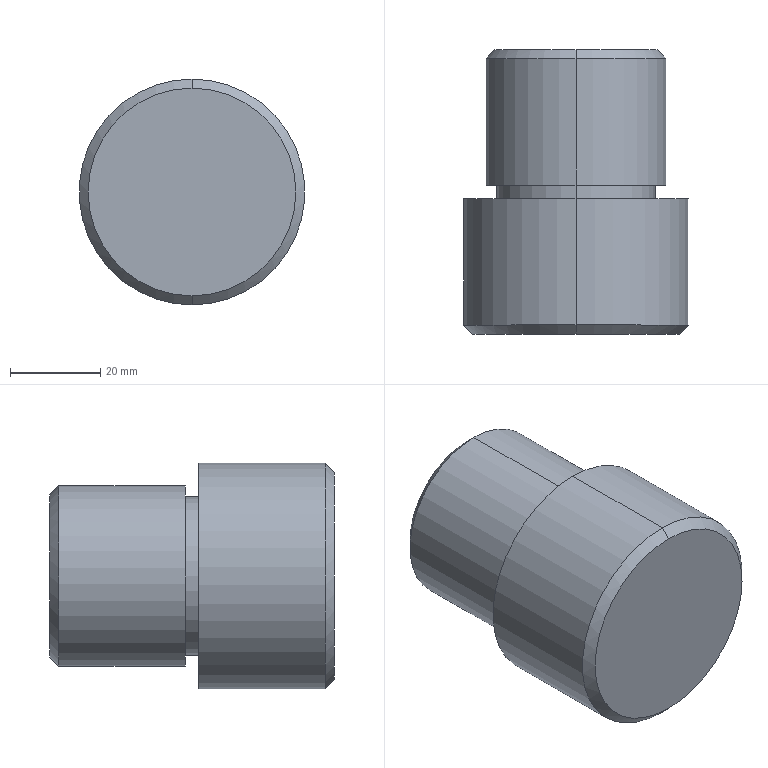Part | SolidWorks | features Chamfer 2, Revolution 1 | 1 solid | 14 faces | box 50 x 63 x 50 mm | volume 98942 mm3 | cylinder 6 | cone 4 | plane 4 | commonest cylinder face diameters 35 x2 40 x2 50 x2
STEP:
#1=CARTESIAN_POINT('',(0.,-35.605,-23.));
#2=VERTEX_POINT('',#1);
#3=CARTESIAN_POINT('',(0.,-35.605,23.));
#4=VERTEX_POINT('',#3);
#5=CARTESIAN_POINT('',(0.,-35.605,0.));
#6=DIRECTION('',(0.,-1.,0.));
#7=DIRECTION('',(0.,0.,1.));
#8=AXIS2_PLACEMENT_3D('',#5,#6,#7);
#9=CIRCLE('',#8,23.);
#10=EDGE_CURVE('',#2,#4,#9,.T.);
#11=ORIENTED_EDGE('',*,*,#10,.F.);
#12=CARTESIAN_POINT('',(0.,-33.605,-25.));
#13=VERTEX_POINT('',#12);
#14=CARTESIAN_POINT('',(0.,-33.605,-25.));
#15=DIRECTION('',(0.,0.7071,-0.7071));
#16=VECTOR('',#15,1000.);
#17=LINE('',#14,#16);
#18=EDGE_CURVE('',#2,#13,#17,.T.);
#19=ORIENTED_EDGE('',*,*,#18,.T.);
#20=CARTESIAN_POINT('',(0.,-33.605,25.));
#21=VERTEX_POINT('',#20);
#22=CARTESIAN_POINT('',(0.,-33.605,0.));
#23=DIRECTION('',(0.,1.,0.));
#24=DIRECTION('',(0.,0.,1.));
#25=AXIS2_PLACEMENT_3D('',#22,#23,#24);
#26=CIRCLE('',#25,25.);
#27=EDGE_CURVE('',#21,#13,#26,.T.);
#28=ORIENTED_EDGE('',*,*,#27,.F.);
#29=CARTESIAN_POINT('',(0.,-33.605,25.));
#30=DIRECTION('',(0.,0.7071,0.7071));
#31=VECTOR('',#30,1000.);
#32=LINE('',#29,#31);
#33=EDGE_CURVE('',#4,#21,#32,.T.);
#34=ORIENTED_EDGE('',*,*,#33,.F.);
#35=EDGE_LOOP('',(#11,#19,#28,#34));
#36=FACE_OUTER_BOUND('',#35,.T.);
#37=CARTESIAN_POINT('',(0.,-33.605,0.));
#38=DIRECTION('',(0.,1.,0.));
#39=DIRECTION('',(0.,0.,1.));
#40=AXIS2_PLACEMENT_3D('',#37,#38,#39);
#41=CONICAL_SURFACE('',#40,25.,0.7854);
#42=ADVANCED_FACE('',(#36),#41,.T.);
#43=CARTESIAN_POINT('',(0.,27.395,18.));
#44=VERTEX_POINT('',#43);
#45=CARTESIAN_POINT('',(0.,27.395,-18.));
#46=VERTEX_POINT('',#45);
#47=CARTESIAN_POINT('',(0.,27.395,0.));
#48=DIRECTION('',(0.,1.,0.));
#49=DIRECTION('',(0.,0.,1.));
#50=AXIS2_PLACEMENT_3D('',#47,#48,#49);
#51=CIRCLE('',#50,18.);
#52=EDGE_CURVE('',#44,#46,#51,.T.);
#53=ORIENTED_EDGE('',*,*,#52,.F.);
#54=CARTESIAN_POINT('',(0.,25.395,20.));
#55=VERTEX_POINT('',#54);
#56=CARTESIAN_POINT('',(0.,27.395,18.));
#57=DIRECTION('',(0.,-0.7071,0.7071));
#58=VECTOR('',#57,1000.);
#59=LINE('',#56,#58);
#60=EDGE_CURVE('',#44,#55,#59,.T.);
#61=ORIENTED_EDGE('',*,*,#60,.T.);
#62=CARTESIAN_POINT('',(0.,25.395,-20.));
#63=VERTEX_POINT('',#62);
#64=CARTESIAN_POINT('',(0.,25.395,0.));
#65=DIRECTION('',(0.,-1.,0.));
#66=DIRECTION('',(0.,0.,1.));
#67=AXIS2_PLACEMENT_3D('',#64,#65,#66);
#68=CIRCLE('',#67,20.);
#69=EDGE_CURVE('',#63,#55,#68,.T.);
#70=ORIENTED_EDGE('',*,*,#69,.F.);
#71=CARTESIAN_POINT('',(0.,27.395,-18.));
#72=DIRECTION('',(0.,-0.7071,-0.7071));
#73=VECTOR('',#72,1000.);
#74=LINE('',#71,#73);
#75=EDGE_CURVE('',#46,#63,#74,.T.);
#76=ORIENTED_EDGE('',*,*,#75,.F.);
#77=EDGE_LOOP('',(#53,#61,#70,#76));
#78=FACE_OUTER_BOUND('',#77,.T.);
#79=CARTESIAN_POINT('',(0.,27.395,0.));
#80=DIRECTION('',(0.,-1.,0.));
#81=DIRECTION('',(0.,0.,-1.));
#82=AXIS2_PLACEMENT_3D('',#79,#80,#81);
#83=CONICAL_SURFACE('',#82,18.,0.7854);
#84=ADVANCED_FACE('',(#78),#83,.T.);
#85=CARTESIAN_POINT('',(0.,-5.605,17.5));
#86=VERTEX_POINT('',#85);
#87=CARTESIAN_POINT('',(0.,-5.605,-17.5));
#88=VERTEX_POINT('',#87);
#89=CARTESIAN_POINT('',(0.,-5.605,0.));
#90=DIRECTION('',(0.,1.,0.));
#91=DIRECTION('',(0.,0.,1.));
#92=AXIS2_PLACEMENT_3D('',#89,#90,#91);
#93=CIRCLE('',#92,17.5);
#94=EDGE_CURVE('',#86,#88,#93,.T.);
#95=ORIENTED_EDGE('',*,*,#94,.T.);
#96=CARTESIAN_POINT('',(0.,-2.605,-17.5));
#97=VERTEX_POINT('',#96);
#98=CARTESIAN_POINT('',(0.,37.5,-17.5));
#99=DIRECTION('',(0.,1.,0.));
#100=VECTOR('',#99,1000.);
#101=LINE('',#98,#100);
#102=EDGE_CURVE('',#88,#97,#101,.T.);
#103=ORIENTED_EDGE('',*,*,#102,.T.);
#104=CARTESIAN_POINT('',(0.,-2.605,17.5));
#105=VERTEX_POINT('',#104);
#106=CARTESIAN_POINT('',(0.,-2.605,0.));
#107=DIRECTION('',(0.,1.,0.));
#108=DIRECTION('',(0.,0.,1.));
#109=AXIS2_PLACEMENT_3D('',#106,#107,#108);
#110=CIRCLE('',#109,17.5);
#111=EDGE_CURVE('',#105,#97,#110,.T.);
#112=ORIENTED_EDGE('',*,*,#111,.F.);
#113=CARTESIAN_POINT('',(0.,37.5,17.5));
#114=DIRECTION('',(0.,1.,0.));
#115=VECTOR('',#114,1000.);
#116=LINE('',#113,#115);
#117=EDGE_CURVE('',#86,#105,#116,.T.);
#118=ORIENTED_EDGE('',*,*,#117,.F.);
#119=EDGE_LOOP('',(#95,#103,#112,#118));
#120=FACE_OUTER_BOUND('',#119,.T.);
#121=CARTESIAN_POINT('',(0.,37.5,0.));
#122=DIRECTION('',(0.,1.,0.));
#123=DIRECTION('',(0.,0.,1.));
#124=AXIS2_PLACEMENT_3D('',#121,#122,#123);
#125=CYLINDRICAL_SURFACE('',#124,17.5);
#126=ADVANCED_FACE('',(#120),#125,.T.);
#127=CARTESIAN_POINT('',(0.,-2.605,20.));
#128=VERTEX_POINT('',#127);
#129=CARTESIAN_POINT('',(0.,-2.605,-20.));
#130=VERTEX_POINT('',#129);
#131=CARTESIAN_POINT('',(0.,-2.605,0.));
#132=DIRECTION('',(0.,1.,0.));
#133=DIRECTION('',(0.,0.,1.));
#134=AXIS2_PLACEMENT_3D('',#131,#132,#133);
#135=CIRCLE('',#134,20.);
#136=EDGE_CURVE('',#128,#130,#135,.T.);
#137=ORIENTED_EDGE('',*,*,#136,.T.);
#138=CARTESIAN_POINT('',(0.,37.5,-20.));
#139=DIRECTION('',(0.,1.,0.));
#140=VECTOR('',#139,1000.);
#141=LINE('',#138,#140);
#142=EDGE_CURVE('',#130,#63,#141,.T.);
#143=ORIENTED_EDGE('',*,*,#142,.T.);
#144=ORIENTED_EDGE('',*,*,#69,.T.);
#145=CARTESIAN_POINT('',(0.,37.5,20.));
#146=DIRECTION('',(0.,1.,0.));
#147=VECTOR('',#146,1000.);
#148=LINE('',#145,#147);
#149=EDGE_CURVE('',#128,#55,#148,.T.);
#150=ORIENTED_EDGE('',*,*,#149,.F.);
#151=EDGE_LOOP('',(#137,#143,#144,#150));
#152=FACE_OUTER_BOUND('',#151,.T.);
#153=CARTESIAN_POINT('',(0.,37.5,0.));
#154=DIRECTION('',(0.,1.,0.));
#155=DIRECTION('',(0.,0.,1.));
#156=AXIS2_PLACEMENT_3D('',#153,#154,#155);
#157=CYLINDRICAL_SURFACE('',#156,20.);
#158=ADVANCED_FACE('',(#152),#157,.T.);
#159=ORIENTED_EDGE('',*,*,#27,.T.);
#160=CARTESIAN_POINT('',(0.,-5.605,-25.));
#161=VERTEX_POINT('',#160);
#162=CARTESIAN_POINT('',(0.,37.5,-25.));
#163=DIRECTION('',(0.,1.,0.));
#164=VECTOR('',#163,1000.);
#165=LINE('',#162,#164);
#166=EDGE_CURVE('',#13,#161,#165,.T.);
#167=ORIENTED_EDGE('',*,*,#166,.T.);
#168=CARTESIAN_POINT('',(0.,-5.605,25.));
#169=VERTEX_POINT('',#168);
#170=CARTESIAN_POINT('',(0.,-5.605,0.));
#171=DIRECTION('',(0.,1.,0.));
#172=DIRECTION('',(0.,0.,1.));
#173=AXIS2_PLACEMENT_3D('',#170,#171,#172);
#174=CIRCLE('',#173,25.);
#175=EDGE_CURVE('',#169,#161,#174,.T.);
#176=ORIENTED_EDGE('',*,*,#175,.F.);
#177=CARTESIAN_POINT('',(0.,37.5,25.));
#178=DIRECTION('',(0.,1.,0.));
#179=VECTOR('',#178,1000.);
#180=LINE('',#177,#179);
#181=EDGE_CURVE('',#21,#169,#180,.T.);
#182=ORIENTED_EDGE('',*,*,#181,.F.);
#183=EDGE_LOOP('',(#159,#167,#176,#182));
#184=FACE_OUTER_BOUND('',#183,.T.);
#185=CARTESIAN_POINT('',(0.,37.5,0.));
#186=DIRECTION('',(0.,1.,0.));
#187=DIRECTION('',(0.,0.,1.));
#188=AXIS2_PLACEMENT_3D('',#185,#186,#187);
#189=CYLINDRICAL_SURFACE('',#188,25.);
#190=ADVANCED_FACE('',(#184),#189,.T.);
#191=ORIENTED_EDGE('',*,*,#175,.T.);
#192=CARTESIAN_POINT('',(0.,-5.605,0.));
#193=DIRECTION('',(0.,1.,0.));
#194=DIRECTION('',(0.,0.,1.));
#195=AXIS2_PLACEMENT_3D('',#192,#193,#194);
#196=CIRCLE('',#195,25.);
#197=EDGE_CURVE('',#161,#169,#196,.T.);
#198=ORIENTED_EDGE('',*,*,#197,.T.);
#199=EDGE_LOOP('',(#191,#198));
#200=FACE_OUTER_BOUND('',#199,.T.);
#201=ORIENTED_EDGE('',*,*,#94,.F.);
#202=CARTESIAN_POINT('',(0.,-5.605,0.));
#203=DIRECTION('',(0.,1.,0.));
#204=DIRECTION('',(0.,0.,1.));
#205=AXIS2_PLACEMENT_3D('',#202,#203,#204);
#206=CIRCLE('',#205,17.5);
#207=EDGE_CURVE('',#88,#86,#206,.T.);
#208=ORIENTED_EDGE('',*,*,#207,.F.);
#209=EDGE_LOOP('',(#201,#208));
#210=FACE_BOUND('',#209,.T.);
#211=CARTESIAN_POINT('',(0.,-5.605,0.));
#212=DIRECTION('',(0.,1.,0.));
#213=DIRECTION('',(0.,0.,1.));
#214=AXIS2_PLACEMENT_3D('',#211,#212,#213);
#215=PLANE('',#214);
#216=ADVANCED_FACE('',(#200,#210),#215,.T.);
#217=ORIENTED_EDGE('',*,*,#166,.F.);
#218=CARTESIAN_POINT('',(0.,-33.605,0.));
#219=DIRECTION('',(0.,1.,0.));
#220=DIRECTION('',(0.,0.,1.));
#221=AXIS2_PLACEMENT_3D('',#218,#219,#220);
#222=CIRCLE('',#221,25.);
#223=EDGE_CURVE('',#13,#21,#222,.T.);
#224=ORIENTED_EDGE('',*,*,#223,.T.);
#225=ORIENTED_EDGE('',*,*,#181,.T.);
#226=ORIENTED_EDGE('',*,*,#197,.F.);
#227=EDGE_LOOP('',(#217,#224,#225,#226));
#228=FACE_OUTER_BOUND('',#227,.T.);
#229=CARTESIAN_POINT('',(0.,37.5,0.));
#230=DIRECTION('',(0.,1.,0.));
#231=DIRECTION('',(0.,0.,1.));
#232=AXIS2_PLACEMENT_3D('',#229,#230,#231);
#233=CYLINDRICAL_SURFACE('',#232,25.);
#234=ADVANCED_FACE('',(#228),#233,.T.);
#235=CARTESIAN_POINT('',(0.,-35.605,0.));
#236=DIRECTION('',(0.,-1.,0.));
#237=DIRECTION('',(0.,0.,1.));
#238=AXIS2_PLACEMENT_3D('',#235,#236,#237);
#239=CIRCLE('',#238,23.);
#240=EDGE_CURVE('',#4,#2,#239,.T.);
#241=ORIENTED_EDGE('',*,*,#240,.T.);
#242=ORIENTED_EDGE('',*,*,#10,.T.);
#243=EDGE_LOOP('',(#241,#242));
#244=FACE_OUTER_BOUND('',#243,.T.);
#245=CARTESIAN_POINT('',(0.,-35.605,0.));
#246=DIRECTION('',(0.,1.,0.));
#247=DIRECTION('',(0.,0.,1.));
#248=AXIS2_PLACEMENT_3D('',#245,#246,#247);
#249=PLANE('',#248);
#250=ADVANCED_FACE('',(#244),#249,.F.);
#251=CARTESIAN_POINT('',(0.,27.395,0.));
#252=DIRECTION('',(0.,1.,0.));
#253=DIRECTION('',(0.,0.,1.));
#254=AXIS2_PLACEMENT_3D('',#251,#252,#253);
#255=CIRCLE('',#254,18.);
#256=EDGE_CURVE('',#46,#44,#255,.T.);
#257=ORIENTED_EDGE('',*,*,#256,.T.);
#258=ORIENTED_EDGE('',*,*,#52,.T.);
#259=EDGE_LOOP('',(#257,#258));
#260=FACE_OUTER_BOUND('',#259,.T.);
#261=CARTESIAN_POINT('',(0.,27.395,0.));
#262=DIRECTION('',(0.,1.,0.));
#263=DIRECTION('',(0.,0.,1.));
#264=AXIS2_PLACEMENT_3D('',#261,#262,#263);
#265=PLANE('',#264);
#266=ADVANCED_FACE('',(#260),#265,.T.);
#267=ORIENTED_EDGE('',*,*,#142,.F.);
#268=CARTESIAN_POINT('',(0.,-2.605,0.));
#269=DIRECTION('',(0.,1.,0.));
#270=DIRECTION('',(0.,0.,1.));
#271=AXIS2_PLACEMENT_3D('',#268,#269,#270);
#272=CIRCLE('',#271,20.);
#273=EDGE_CURVE('',#130,#128,#272,.T.);
#274=ORIENTED_EDGE('',*,*,#273,.T.);
#275=ORIENTED_EDGE('',*,*,#149,.T.);
#276=CARTESIAN_POINT('',(0.,25.395,0.));
#277=DIRECTION('',(0.,-1.,0.));
#278=DIRECTION('',(0.,0.,1.));
#279=AXIS2_PLACEMENT_3D('',#276,#277,#278);
#280=CIRCLE('',#279,20.);
#281=EDGE_CURVE('',#55,#63,#280,.T.);
#282=ORIENTED_EDGE('',*,*,#281,.T.);
#283=EDGE_LOOP('',(#267,#274,#275,#282));
#284=FACE_OUTER_BOUND('',#283,.T.);
#285=CARTESIAN_POINT('',(0.,37.5,0.));
#286=DIRECTION('',(0.,1.,0.));
#287=DIRECTION('',(0.,0.,1.));
#288=AXIS2_PLACEMENT_3D('',#285,#286,#287);
#289=CYLINDRICAL_SURFACE('',#288,20.);
#290=ADVANCED_FACE('',(#284),#289,.T.);
#291=ORIENTED_EDGE('',*,*,#136,.F.);
#292=ORIENTED_EDGE('',*,*,#273,.F.);
#293=EDGE_LOOP('',(#291,#292));
#294=FACE_OUTER_BOUND('',#293,.T.);
#295=ORIENTED_EDGE('',*,*,#111,.T.);
#296=CARTESIAN_POINT('',(0.,-2.605,0.));
#297=DIRECTION('',(0.,1.,0.));
#298=DIRECTION('',(0.,0.,1.));
#299=AXIS2_PLACEMENT_3D('',#296,#297,#298);
#300=CIRCLE('',#299,17.5);
#301=EDGE_CURVE('',#97,#105,#300,.T.);
#302=ORIENTED_EDGE('',*,*,#301,.T.);
#303=EDGE_LOOP('',(#295,#302));
#304=FACE_BOUND('',#303,.T.);
#305=CARTESIAN_POINT('',(0.,-2.605,0.));
#306=DIRECTION('',(0.,1.,0.));
#307=DIRECTION('',(0.,0.,1.));
#308=AXIS2_PLACEMENT_3D('',#305,#306,#307);
#309=PLANE('',#308);
#310=ADVANCED_FACE('',(#294,#304),#309,.F.);
#311=ORIENTED_EDGE('',*,*,#102,.F.);
#312=ORIENTED_EDGE('',*,*,#207,.T.);
#313=ORIENTED_EDGE('',*,*,#117,.T.);
#314=ORIENTED_EDGE('',*,*,#301,.F.);
#315=EDGE_LOOP('',(#311,#312,#313,#314));
#316=FACE_OUTER_BOUND('',#315,.T.);
#317=CARTESIAN_POINT('',(0.,37.5,0.));
#318=DIRECTION('',(0.,1.,0.));
#319=DIRECTION('',(0.,0.,1.));
#320=AXIS2_PLACEMENT_3D('',#317,#318,#319);
#321=CYLINDRICAL_SURFACE('',#320,17.5);
#322=ADVANCED_FACE('',(#316),#321,.T.);
#323=ORIENTED_EDGE('',*,*,#60,.F.);
#324=ORIENTED_EDGE('',*,*,#256,.F.);
#325=ORIENTED_EDGE('',*,*,#75,.T.);
#326=ORIENTED_EDGE('',*,*,#281,.F.);
#327=EDGE_LOOP('',(#323,#324,#325,#326));
#328=FACE_OUTER_BOUND('',#327,.T.);
#329=CARTESIAN_POINT('',(0.,27.395,0.));
#330=DIRECTION('',(0.,-1.,0.));
#331=DIRECTION('',(0.,0.,-1.));
#332=AXIS2_PLACEMENT_3D('',#329,#330,#331);
#333=CONICAL_SURFACE('',#332,18.,0.7854);
#334=ADVANCED_FACE('',(#328),#333,.T.);
#335=ORIENTED_EDGE('',*,*,#18,.F.);
#336=ORIENTED_EDGE('',*,*,#240,.F.);
#337=ORIENTED_EDGE('',*,*,#33,.T.);
#338=ORIENTED_EDGE('',*,*,#223,.F.);
#339=EDGE_LOOP('',(#335,#336,#337,#338));
#340=FACE_OUTER_BOUND('',#339,.T.);
#341=CARTESIAN_POINT('',(0.,-33.605,0.));
#342=DIRECTION('',(0.,1.,0.));
#343=DIRECTION('',(0.,0.,1.));
#344=AXIS2_PLACEMENT_3D('',#341,#342,#343);
#345=CONICAL_SURFACE('',#344,25.,0.7854);
#346=ADVANCED_FACE('',(#340),#345,.T.);
#347=CLOSED_SHELL('',(#42,#84,#126,#158,#190,#216,#234,#250,#266,#290,#310,#322,#334,#346));
#348=MANIFOLD_SOLID_BREP('',#347);
#349=CARTESIAN_POINT('',(0.,0.,0.));
#350=DIRECTION('',(0.,0.,1.));
#351=DIRECTION('',(1.,0.,0.));
#352=AXIS2_PLACEMENT_3D('',#349,#350,#351);
#353=(LENGTH_UNIT()NAMED_UNIT(*)SI_UNIT(.MILLI.,.METRE.));
#354=UNCERTAINTY_MEASURE_WITH_UNIT(LENGTH_MEASURE(0.00001),#353,'','');
#355=(NAMED_UNIT(*)PLANE_ANGLE_UNIT()SI_UNIT($,.RADIAN.));
#356=(NAMED_UNIT(*)SI_UNIT($,.STERADIAN.)SOLID_ANGLE_UNIT());
#357=(GEOMETRIC_REPRESENTATION_CONTEXT(3)GLOBAL_UNCERTAINTY_ASSIGNED_CONTEXT((#354))GLOBAL_UNIT_ASSIGNED_CONTEXT((#353,#355,#356))REPRESENTATION_CONTEXT('',''));
#358=ADVANCED_BREP_SHAPE_REPRESENTATION('',(#348,#352),#357);